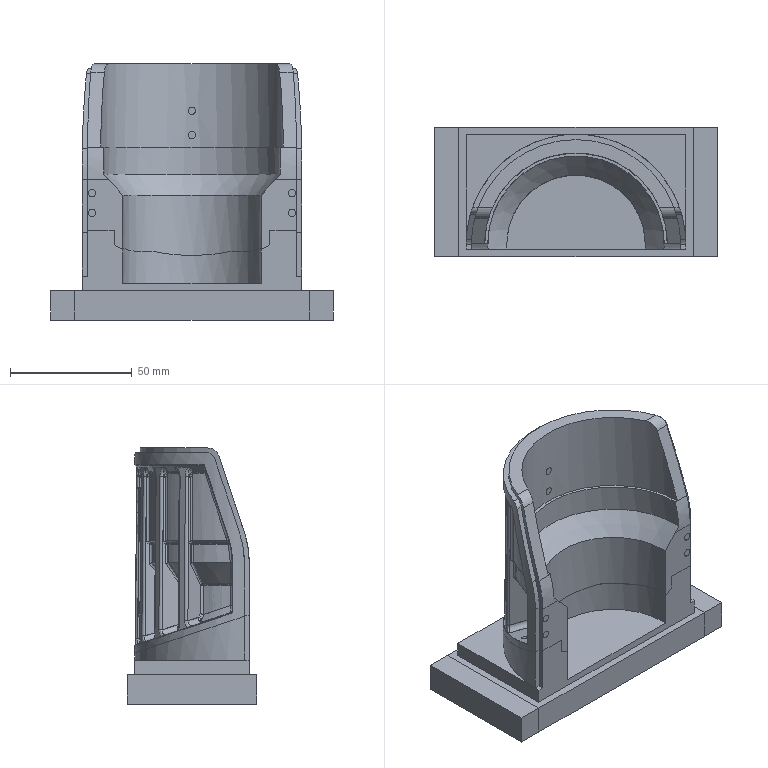Part | 5 solids | 744 faces | box 116 x 53 x 105 mm | volume 244809 mm3 | spline 299 | cylinder 180 | plane 136 | cone 60 | sphere 45 | torus 24 | commonest cylinder face diameters 2 x46 4 x28 84 x20 66 x16 82 x16 3 x6